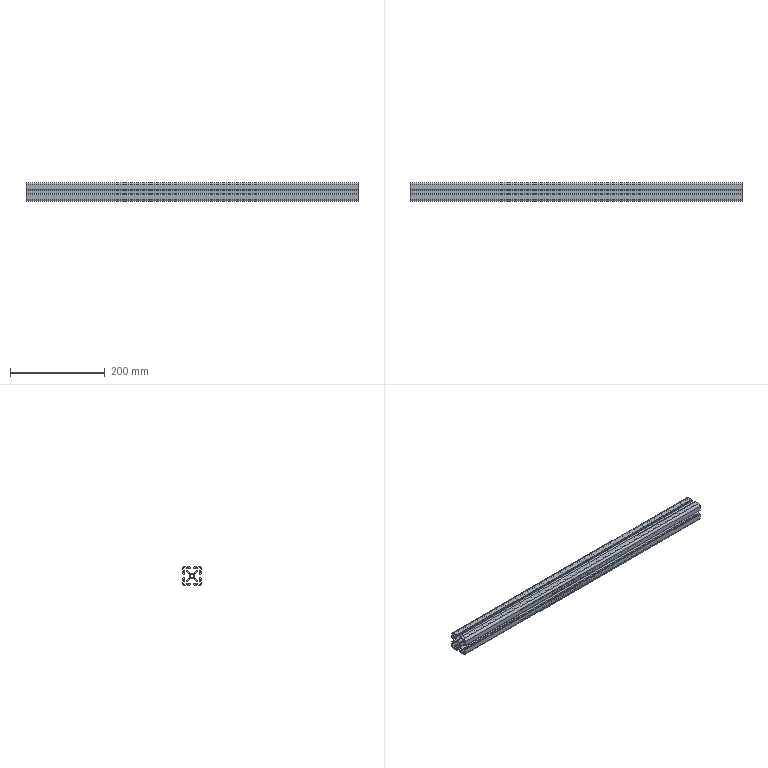Part | STEP file | MK-8-4040C-L-00 profile 4040C standard type 700mm | 1 solid | 188 faces | box 700 x 40 x 40 mm | volume 334774 mm3 | cylinder 94 | plane 94 | commonest cylinder face diameters 0.6 x30 2 x28 4 x16 0.4 x8 6 x4 9 x4